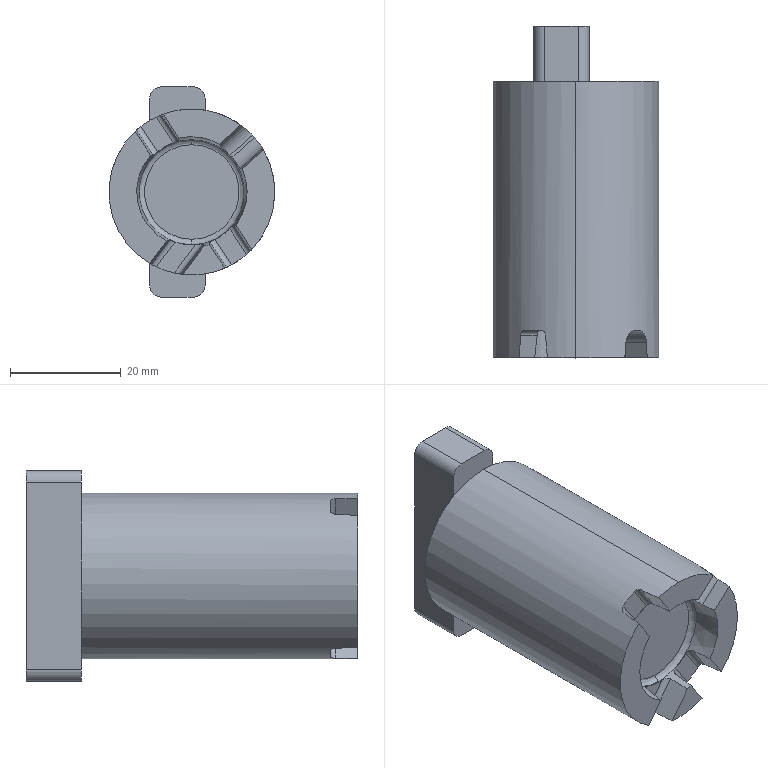Part | STEP file | 1 solid | 44 faces | box 30 x 60 x 38 mm | volume 36750 mm3 | plane 26 | cylinder 14 | torus 2 | cone 2 | commonest cylinder face diameters 2 x6 4 x4 5 x2 30 x2